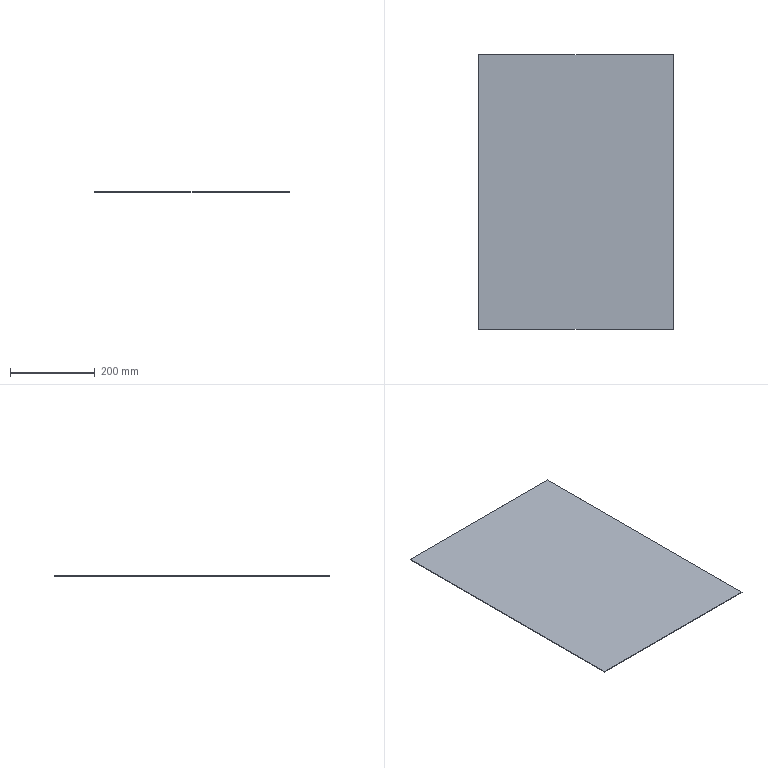Part | STEP file | B1-033 | 1 solid | 6 faces | box 460 x 650 x 1.5 mm | volume 448500 mm3 | plane 6
STEP:
#1=CARTESIAN_POINT('',(0.,0.,0.));
#2=DIRECTION('',(0.,0.,1.));
#3=DIRECTION('',(1.,0.,0.));
#4=AXIS2_PLACEMENT_3D('',#1,#2,#3);
#5=CARTESIAN_POINT('',(230.,-325.,0.));
#6=VERTEX_POINT('',#5);
#7=CARTESIAN_POINT('',(230.,325.,0.));
#8=VERTEX_POINT('',#7);
#9=CARTESIAN_POINT('',(230.,325.,0.));
#10=DIRECTION('',(0.,1.,0.));
#11=VECTOR('',#10,1.);
#12=LINE('',#9,#11);
#13=CARTESIAN_POINT('',(230.,325.,1.5));
#14=DIRECTION('',(-1.,0.,0.));
#15=DIRECTION('',(0.,0.,1.));
#16=AXIS2_PLACEMENT_3D('',#13,#14,#15);
#17=PLANE('',#16);
#18=CARTESIAN_POINT('',(-1.5,0.));
#19=DIRECTION('',(0.,1.));
#20=VECTOR('',#19,1.);
#21=LINE('',#18,#20);
#22=(GEOMETRIC_REPRESENTATION_CONTEXT(2)PARAMETRIC_REPRESENTATION_CONTEXT()REPRESENTATION_CONTEXT('',''));
#23=DEFINITIONAL_REPRESENTATION('',(#21),#22);
#24=PCURVE('',#17,#23);
#25=CARTESIAN_POINT('',(0.,0.,0.));
#26=DIRECTION('',(0.,0.,1.));
#27=DIRECTION('',(1.,0.,0.));
#28=AXIS2_PLACEMENT_3D('',#25,#26,#27);
#29=PLANE('',#28);
#30=CARTESIAN_POINT('',(230.,325.));
#31=DIRECTION('',(0.,1.));
#32=VECTOR('',#31,1.);
#33=LINE('',#30,#32);
#34=(GEOMETRIC_REPRESENTATION_CONTEXT(2)PARAMETRIC_REPRESENTATION_CONTEXT()REPRESENTATION_CONTEXT('',''));
#35=DEFINITIONAL_REPRESENTATION('',(#33),#34);
#36=PCURVE('',#29,#35);
#37=SURFACE_CURVE('',#12,(#24,#36),.PCURVE_S1.);
#38=EDGE_CURVE('',#6,#8,#37,.T.);
#39=ORIENTED_EDGE('',*,*,#38,.T.);
#40=CARTESIAN_POINT('',(230.,325.,1.5));
#41=VERTEX_POINT('',#40);
#42=CARTESIAN_POINT('',(230.,325.,1.5));
#43=DIRECTION('',(0.,0.,-1.));
#44=VECTOR('',#43,1.);
#45=LINE('',#42,#44);
#46=CARTESIAN_POINT('',(0.,0.));
#47=DIRECTION('',(-1.,0.));
#48=VECTOR('',#47,1.);
#49=LINE('',#46,#48);
#50=(GEOMETRIC_REPRESENTATION_CONTEXT(2)PARAMETRIC_REPRESENTATION_CONTEXT()REPRESENTATION_CONTEXT('',''));
#51=DEFINITIONAL_REPRESENTATION('',(#49),#50);
#52=PCURVE('',#17,#51);
#53=CARTESIAN_POINT('',(-230.,325.,1.5));
#54=DIRECTION('',(0.,-1.,0.));
#55=DIRECTION('',(0.,0.,-1.));
#56=AXIS2_PLACEMENT_3D('',#53,#54,#55);
#57=PLANE('',#56);
#58=CARTESIAN_POINT('',(0.,460.));
#59=DIRECTION('',(1.,0.));
#60=VECTOR('',#59,1.);
#61=LINE('',#58,#60);
#62=(GEOMETRIC_REPRESENTATION_CONTEXT(2)PARAMETRIC_REPRESENTATION_CONTEXT()REPRESENTATION_CONTEXT('',''));
#63=DEFINITIONAL_REPRESENTATION('',(#61),#62);
#64=PCURVE('',#57,#63);
#65=SURFACE_CURVE('',#45,(#52,#64),.PCURVE_S1.);
#66=EDGE_CURVE('',#41,#8,#65,.T.);
#67=ORIENTED_EDGE('',*,*,#66,.F.);
#68=CARTESIAN_POINT('',(230.,-325.,1.5));
#69=VERTEX_POINT('',#68);
#70=CARTESIAN_POINT('',(230.,325.,1.5));
#71=DIRECTION('',(0.,1.,0.));
#72=VECTOR('',#71,1.);
#73=LINE('',#70,#72);
#74=CARTESIAN_POINT('',(0.,0.));
#75=DIRECTION('',(0.,1.));
#76=VECTOR('',#75,1.);
#77=LINE('',#74,#76);
#78=(GEOMETRIC_REPRESENTATION_CONTEXT(2)PARAMETRIC_REPRESENTATION_CONTEXT()REPRESENTATION_CONTEXT('',''));
#79=DEFINITIONAL_REPRESENTATION('',(#77),#78);
#80=PCURVE('',#17,#79);
#81=CARTESIAN_POINT('',(0.,0.,1.5));
#82=DIRECTION('',(0.,0.,1.));
#83=DIRECTION('',(1.,0.,0.));
#84=AXIS2_PLACEMENT_3D('',#81,#82,#83);
#85=PLANE('',#84);
#86=CARTESIAN_POINT('',(230.,325.));
#87=DIRECTION('',(0.,1.));
#88=VECTOR('',#87,1.);
#89=LINE('',#86,#88);
#90=(GEOMETRIC_REPRESENTATION_CONTEXT(2)PARAMETRIC_REPRESENTATION_CONTEXT()REPRESENTATION_CONTEXT('',''));
#91=DEFINITIONAL_REPRESENTATION('',(#89),#90);
#92=PCURVE('',#85,#91);
#93=SURFACE_CURVE('',#73,(#80,#92),.PCURVE_S1.);
#94=EDGE_CURVE('',#69,#41,#93,.T.);
#95=ORIENTED_EDGE('',*,*,#94,.F.);
#96=CARTESIAN_POINT('',(230.,-325.,1.5));
#97=DIRECTION('',(0.,0.,-1.));
#98=VECTOR('',#97,1.);
#99=LINE('',#96,#98);
#100=CARTESIAN_POINT('',(0.,-650.));
#101=DIRECTION('',(-1.,0.));
#102=VECTOR('',#101,1.);
#103=LINE('',#100,#102);
#104=(GEOMETRIC_REPRESENTATION_CONTEXT(2)PARAMETRIC_REPRESENTATION_CONTEXT()REPRESENTATION_CONTEXT('',''));
#105=DEFINITIONAL_REPRESENTATION('',(#103),#104);
#106=PCURVE('',#17,#105);
#107=CARTESIAN_POINT('',(-230.,-325.,1.5));
#108=DIRECTION('',(0.,1.,0.));
#109=DIRECTION('',(0.,0.,1.));
#110=AXIS2_PLACEMENT_3D('',#107,#108,#109);
#111=PLANE('',#110);
#112=CARTESIAN_POINT('',(0.,460.));
#113=DIRECTION('',(-1.,0.));
#114=VECTOR('',#113,1.);
#115=LINE('',#112,#114);
#116=(GEOMETRIC_REPRESENTATION_CONTEXT(2)PARAMETRIC_REPRESENTATION_CONTEXT()REPRESENTATION_CONTEXT('',''));
#117=DEFINITIONAL_REPRESENTATION('',(#115),#116);
#118=PCURVE('',#111,#117);
#119=SURFACE_CURVE('',#99,(#106,#118),.PCURVE_S1.);
#120=EDGE_CURVE('',#69,#6,#119,.T.);
#121=ORIENTED_EDGE('',*,*,#120,.T.);
#122=EDGE_LOOP('',(#39,#67,#95,#121));
#123=FACE_BOUND('',#122,.T.);
#124=ADVANCED_FACE('',(#123),#17,.F.);
#125=CARTESIAN_POINT('',(-230.,325.,0.));
#126=VERTEX_POINT('',#125);
#127=CARTESIAN_POINT('',(-230.,325.,0.));
#128=DIRECTION('',(-1.,0.,0.));
#129=VECTOR('',#128,1.);
#130=LINE('',#127,#129);
#131=CARTESIAN_POINT('',(1.5,0.));
#132=DIRECTION('',(0.,-1.));
#133=VECTOR('',#132,1.);
#134=LINE('',#131,#133);
#135=(GEOMETRIC_REPRESENTATION_CONTEXT(2)PARAMETRIC_REPRESENTATION_CONTEXT()REPRESENTATION_CONTEXT('',''));
#136=DEFINITIONAL_REPRESENTATION('',(#134),#135);
#137=PCURVE('',#57,#136);
#138=CARTESIAN_POINT('',(-230.,325.));
#139=DIRECTION('',(-1.,0.));
#140=VECTOR('',#139,1.);
#141=LINE('',#138,#140);
#142=(GEOMETRIC_REPRESENTATION_CONTEXT(2)PARAMETRIC_REPRESENTATION_CONTEXT()REPRESENTATION_CONTEXT('',''));
#143=DEFINITIONAL_REPRESENTATION('',(#141),#142);
#144=PCURVE('',#29,#143);
#145=SURFACE_CURVE('',#130,(#137,#144),.PCURVE_S1.);
#146=EDGE_CURVE('',#8,#126,#145,.T.);
#147=ORIENTED_EDGE('',*,*,#146,.T.);
#148=CARTESIAN_POINT('',(-230.,325.,1.5));
#149=VERTEX_POINT('',#148);
#150=CARTESIAN_POINT('',(-230.,325.,1.5));
#151=DIRECTION('',(0.,0.,-1.));
#152=VECTOR('',#151,1.);
#153=LINE('',#150,#152);
#154=CARTESIAN_POINT('',(0.,0.));
#155=DIRECTION('',(1.,0.));
#156=VECTOR('',#155,1.);
#157=LINE('',#154,#156);
#158=(GEOMETRIC_REPRESENTATION_CONTEXT(2)PARAMETRIC_REPRESENTATION_CONTEXT()REPRESENTATION_CONTEXT('',''));
#159=DEFINITIONAL_REPRESENTATION('',(#157),#158);
#160=PCURVE('',#57,#159);
#161=CARTESIAN_POINT('',(-230.,325.,1.5));
#162=DIRECTION('',(1.,0.,0.));
#163=DIRECTION('',(0.,0.,-1.));
#164=AXIS2_PLACEMENT_3D('',#161,#162,#163);
#165=PLANE('',#164);
#166=CARTESIAN_POINT('',(0.,0.));
#167=DIRECTION('',(1.,0.));
#168=VECTOR('',#167,1.);
#169=LINE('',#166,#168);
#170=(GEOMETRIC_REPRESENTATION_CONTEXT(2)PARAMETRIC_REPRESENTATION_CONTEXT()REPRESENTATION_CONTEXT('',''));
#171=DEFINITIONAL_REPRESENTATION('',(#169),#170);
#172=PCURVE('',#165,#171);
#173=SURFACE_CURVE('',#153,(#160,#172),.PCURVE_S1.);
#174=EDGE_CURVE('',#149,#126,#173,.T.);
#175=ORIENTED_EDGE('',*,*,#174,.F.);
#176=CARTESIAN_POINT('',(-230.,325.,1.5));
#177=DIRECTION('',(-1.,0.,0.));
#178=VECTOR('',#177,1.);
#179=LINE('',#176,#178);
#180=CARTESIAN_POINT('',(0.,0.));
#181=DIRECTION('',(0.,-1.));
#182=VECTOR('',#181,1.);
#183=LINE('',#180,#182);
#184=(GEOMETRIC_REPRESENTATION_CONTEXT(2)PARAMETRIC_REPRESENTATION_CONTEXT()REPRESENTATION_CONTEXT('',''));
#185=DEFINITIONAL_REPRESENTATION('',(#183),#184);
#186=PCURVE('',#57,#185);
#187=CARTESIAN_POINT('',(-230.,325.));
#188=DIRECTION('',(-1.,0.));
#189=VECTOR('',#188,1.);
#190=LINE('',#187,#189);
#191=(GEOMETRIC_REPRESENTATION_CONTEXT(2)PARAMETRIC_REPRESENTATION_CONTEXT()REPRESENTATION_CONTEXT('',''));
#192=DEFINITIONAL_REPRESENTATION('',(#190),#191);
#193=PCURVE('',#85,#192);
#194=SURFACE_CURVE('',#179,(#186,#193),.PCURVE_S1.);
#195=EDGE_CURVE('',#41,#149,#194,.T.);
#196=ORIENTED_EDGE('',*,*,#195,.F.);
#197=ORIENTED_EDGE('',*,*,#66,.T.);
#198=EDGE_LOOP('',(#147,#175,#196,#197));
#199=FACE_BOUND('',#198,.T.);
#200=ADVANCED_FACE('',(#199),#57,.F.);
#201=CARTESIAN_POINT('',(-230.,-325.,0.));
#202=VERTEX_POINT('',#201);
#203=CARTESIAN_POINT('',(-230.,325.,0.));
#204=DIRECTION('',(0.,-1.,0.));
#205=VECTOR('',#204,1.);
#206=LINE('',#203,#205);
#207=CARTESIAN_POINT('',(1.5,0.));
#208=DIRECTION('',(0.,-1.));
#209=VECTOR('',#208,1.);
#210=LINE('',#207,#209);
#211=(GEOMETRIC_REPRESENTATION_CONTEXT(2)PARAMETRIC_REPRESENTATION_CONTEXT()REPRESENTATION_CONTEXT('',''));
#212=DEFINITIONAL_REPRESENTATION('',(#210),#211);
#213=PCURVE('',#165,#212);
#214=CARTESIAN_POINT('',(-230.,325.));
#215=DIRECTION('',(0.,-1.));
#216=VECTOR('',#215,1.);
#217=LINE('',#214,#216);
#218=(GEOMETRIC_REPRESENTATION_CONTEXT(2)PARAMETRIC_REPRESENTATION_CONTEXT()REPRESENTATION_CONTEXT('',''));
#219=DEFINITIONAL_REPRESENTATION('',(#217),#218);
#220=PCURVE('',#29,#219);
#221=SURFACE_CURVE('',#206,(#213,#220),.PCURVE_S1.);
#222=EDGE_CURVE('',#126,#202,#221,.T.);
#223=ORIENTED_EDGE('',*,*,#222,.T.);
#224=CARTESIAN_POINT('',(-230.,-325.,1.5));
#225=VERTEX_POINT('',#224);
#226=CARTESIAN_POINT('',(-230.,-325.,1.5));
#227=DIRECTION('',(0.,0.,-1.));
#228=VECTOR('',#227,1.);
#229=LINE('',#226,#228);
#230=CARTESIAN_POINT('',(0.,-650.));
#231=DIRECTION('',(1.,0.));
#232=VECTOR('',#231,1.);
#233=LINE('',#230,#232);
#234=(GEOMETRIC_REPRESENTATION_CONTEXT(2)PARAMETRIC_REPRESENTATION_CONTEXT()REPRESENTATION_CONTEXT('',''));
#235=DEFINITIONAL_REPRESENTATION('',(#233),#234);
#236=PCURVE('',#165,#235);
#237=CARTESIAN_POINT('',(0.,0.));
#238=DIRECTION('',(-1.,0.));
#239=VECTOR('',#238,1.);
#240=LINE('',#237,#239);
#241=(GEOMETRIC_REPRESENTATION_CONTEXT(2)PARAMETRIC_REPRESENTATION_CONTEXT()REPRESENTATION_CONTEXT('',''));
#242=DEFINITIONAL_REPRESENTATION('',(#240),#241);
#243=PCURVE('',#111,#242);
#244=SURFACE_CURVE('',#229,(#236,#243),.PCURVE_S1.);
#245=EDGE_CURVE('',#225,#202,#244,.T.);
#246=ORIENTED_EDGE('',*,*,#245,.F.);
#247=CARTESIAN_POINT('',(-230.,325.,1.5));
#248=DIRECTION('',(0.,-1.,0.));
#249=VECTOR('',#248,1.);
#250=LINE('',#247,#249);
#251=CARTESIAN_POINT('',(0.,0.));
#252=DIRECTION('',(0.,-1.));
#253=VECTOR('',#252,1.);
#254=LINE('',#251,#253);
#255=(GEOMETRIC_REPRESENTATION_CONTEXT(2)PARAMETRIC_REPRESENTATION_CONTEXT()REPRESENTATION_CONTEXT('',''));
#256=DEFINITIONAL_REPRESENTATION('',(#254),#255);
#257=PCURVE('',#165,#256);
#258=CARTESIAN_POINT('',(-230.,325.));
#259=DIRECTION('',(0.,-1.));
#260=VECTOR('',#259,1.);
#261=LINE('',#258,#260);
#262=(GEOMETRIC_REPRESENTATION_CONTEXT(2)PARAMETRIC_REPRESENTATION_CONTEXT()REPRESENTATION_CONTEXT('',''));
#263=DEFINITIONAL_REPRESENTATION('',(#261),#262);
#264=PCURVE('',#85,#263);
#265=SURFACE_CURVE('',#250,(#257,#264),.PCURVE_S1.);
#266=EDGE_CURVE('',#149,#225,#265,.T.);
#267=ORIENTED_EDGE('',*,*,#266,.F.);
#268=ORIENTED_EDGE('',*,*,#174,.T.);
#269=EDGE_LOOP('',(#223,#246,#267,#268));
#270=FACE_BOUND('',#269,.T.);
#271=ADVANCED_FACE('',(#270),#165,.F.);
#272=CARTESIAN_POINT('',(-230.,-325.,0.));
#273=DIRECTION('',(1.,0.,0.));
#274=VECTOR('',#273,1.);
#275=LINE('',#272,#274);
#276=CARTESIAN_POINT('',(-1.5,0.));
#277=DIRECTION('',(0.,1.));
#278=VECTOR('',#277,1.);
#279=LINE('',#276,#278);
#280=(GEOMETRIC_REPRESENTATION_CONTEXT(2)PARAMETRIC_REPRESENTATION_CONTEXT()REPRESENTATION_CONTEXT('',''));
#281=DEFINITIONAL_REPRESENTATION('',(#279),#280);
#282=PCURVE('',#111,#281);
#283=CARTESIAN_POINT('',(-230.,-325.));
#284=DIRECTION('',(1.,0.));
#285=VECTOR('',#284,1.);
#286=LINE('',#283,#285);
#287=(GEOMETRIC_REPRESENTATION_CONTEXT(2)PARAMETRIC_REPRESENTATION_CONTEXT()REPRESENTATION_CONTEXT('',''));
#288=DEFINITIONAL_REPRESENTATION('',(#286),#287);
#289=PCURVE('',#29,#288);
#290=SURFACE_CURVE('',#275,(#282,#289),.PCURVE_S1.);
#291=EDGE_CURVE('',#202,#6,#290,.T.);
#292=ORIENTED_EDGE('',*,*,#291,.T.);
#293=ORIENTED_EDGE('',*,*,#120,.F.);
#294=CARTESIAN_POINT('',(-230.,-325.,1.5));
#295=DIRECTION('',(1.,0.,0.));
#296=VECTOR('',#295,1.);
#297=LINE('',#294,#296);
#298=CARTESIAN_POINT('',(0.,0.));
#299=DIRECTION('',(0.,1.));
#300=VECTOR('',#299,1.);
#301=LINE('',#298,#300);
#302=(GEOMETRIC_REPRESENTATION_CONTEXT(2)PARAMETRIC_REPRESENTATION_CONTEXT()REPRESENTATION_CONTEXT('',''));
#303=DEFINITIONAL_REPRESENTATION('',(#301),#302);
#304=PCURVE('',#111,#303);
#305=CARTESIAN_POINT('',(-230.,-325.));
#306=DIRECTION('',(1.,0.));
#307=VECTOR('',#306,1.);
#308=LINE('',#305,#307);
#309=(GEOMETRIC_REPRESENTATION_CONTEXT(2)PARAMETRIC_REPRESENTATION_CONTEXT()REPRESENTATION_CONTEXT('',''));
#310=DEFINITIONAL_REPRESENTATION('',(#308),#309);
#311=PCURVE('',#85,#310);
#312=SURFACE_CURVE('',#297,(#304,#311),.PCURVE_S1.);
#313=EDGE_CURVE('',#225,#69,#312,.T.);
#314=ORIENTED_EDGE('',*,*,#313,.F.);
#315=ORIENTED_EDGE('',*,*,#245,.T.);
#316=EDGE_LOOP('',(#292,#293,#314,#315));
#317=FACE_BOUND('',#316,.T.);
#318=ADVANCED_FACE('',(#317),#111,.F.);
#319=ORIENTED_EDGE('',*,*,#94,.T.);
#320=ORIENTED_EDGE('',*,*,#195,.T.);
#321=ORIENTED_EDGE('',*,*,#266,.T.);
#322=ORIENTED_EDGE('',*,*,#313,.T.);
#323=EDGE_LOOP('',(#319,#320,#321,#322));
#324=FACE_BOUND('',#323,.T.);
#325=ADVANCED_FACE('',(#324),#85,.T.);
#326=ORIENTED_EDGE('',*,*,#38,.F.);
#327=ORIENTED_EDGE('',*,*,#291,.F.);
#328=ORIENTED_EDGE('',*,*,#222,.F.);
#329=ORIENTED_EDGE('',*,*,#146,.F.);
#330=EDGE_LOOP('',(#326,#327,#328,#329));
#331=FACE_BOUND('',#330,.T.);
#332=ADVANCED_FACE('',(#331),#29,.F.);
#333=CLOSED_SHELL('',(#124,#200,#271,#318,#325,#332));
#334=MANIFOLD_SOLID_BREP('',#333);
#335=(LENGTH_UNIT()NAMED_UNIT(*)SI_UNIT(.MILLI.,.METRE.));
#336=UNCERTAINTY_MEASURE_WITH_UNIT(LENGTH_MEASURE(0.0000001),#335,'','');
#337=(NAMED_UNIT(*)PLANE_ANGLE_UNIT()SI_UNIT($,.RADIAN.));
#338=(NAMED_UNIT(*)SI_UNIT($,.STERADIAN.)SOLID_ANGLE_UNIT());
#339=(GEOMETRIC_REPRESENTATION_CONTEXT(3)GLOBAL_UNCERTAINTY_ASSIGNED_CONTEXT((#336))GLOBAL_UNIT_ASSIGNED_CONTEXT((#335,#337,#338))REPRESENTATION_CONTEXT('',''));
#340=ADVANCED_BREP_SHAPE_REPRESENTATION('',(#4,#334),#339);